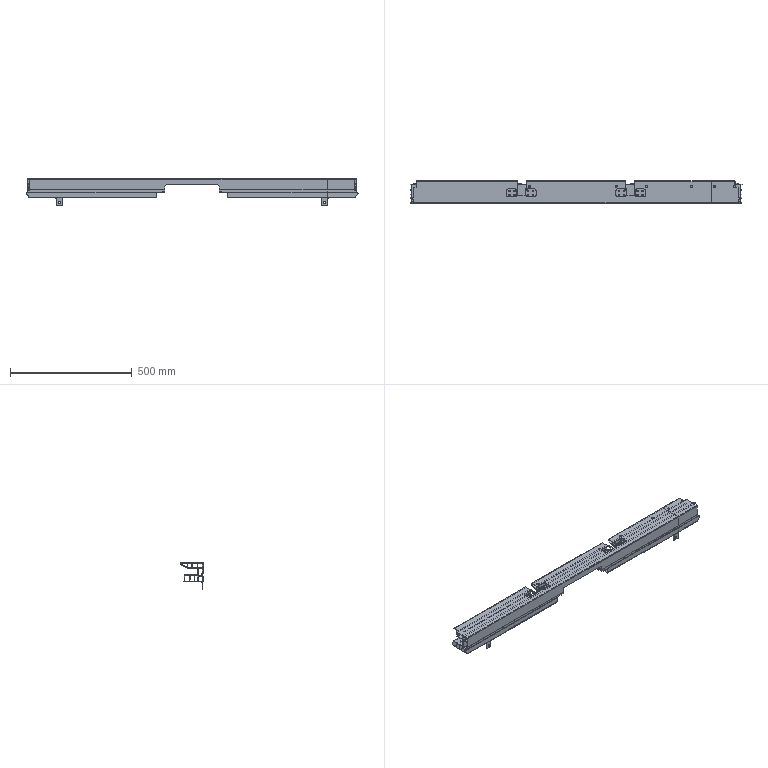NC program | NX | posted with a generic post | part box 1365 x 90.95 x 108.501 mm
Lines 1 to 906 of 22311:
N10 G17 G21 G94 G90
(CAVITY_MILL , TOOL : D16)
N12 T16 M6
N14 G54
N16 G17 G0 G90 X-617.847 Y56.36 B0. C0. S9500 M3
N18 G43 Z30. H16
N20 Z0.503
N22 G94 G1 Z-0.997 F1000.
N24 X-623.563 Y46.46
N26 G2 X-624.429 Y45.96 R1.
N28 G1 X-682.604 F2500.
N30 G3 X-683.352 Y45.208 R0.747
N32 G1 X-683.333 Y41.963
N34 G3 X-682.561 Y41.375 R0.8
N36 G1 X-566.252 Y41.376
N38 G3 X-562.289 Y34.176 R10.036
N40 G1 X-557.527
N42 G2 X-564.365 Y42.175 R8.116
N44 G1 Y45.175
N46 G2 X-557.604 Y53.161 R8.116
N48 G1 X-562.306
N50 G3 X-566.253 Y45.961 R10.036
N52 G1 X-624.429 Y45.96
N54 G2 X-625.295 Y46.46 R1.
N56 G1 X-631.01 Y56.36
N58 Z0.503
N60 G0 X-618.13 Y56.362 Z-0.493
N62 G1 Z-1.993 F1000.
N64 X-623.846 Y46.462
N66 G2 X-624.712 Y45.962 R1.
N68 G1 X-682.604 Y45.961 F2500.
N70 G3 X-683.352 Y45.209 R0.747
N72 G1 X-683.333 Y41.962
N74 G3 X-682.561 Y41.374 R0.8
N76 G1 X-566.819 Y41.375
N78 G3 X-562.862 Y34.175 R10.023
N80 G1 X-558.098
N82 G2 X-564.931 Y42.175 R8.103
N84 G1 Y45.175
N86 G2 X-558.174 Y53.162 R8.103
N88 G1 X-562.879
N90 G3 X-566.82 Y45.962 R10.023
N92 G1 X-624.712
N94 G2 X-625.578 Y46.462 R1.
N96 G1 X-631.294 Y56.362
N98 Z-0.493
N100 G0 X-618.214 Y56.363 Z-1.49
N102 G1 Z-2.99 F1000.
N104 X-623.93 Y46.463
N106 G2 X-624.796 Y45.963 R1.
N108 G1 X-682.604 Y45.962 F2500.
N110 G3 X-683.352 Y45.211 R0.747
N112 G1 X-683.333 Y41.961
N114 G3 X-682.561 Y41.373 R0.8
N116 G1 X-566.986 Y41.374
N118 G3 X-563.03 Y34.174 R10.02
N120 G1 X-558.262
N122 G2 X-565.098 Y42.085 R8.1
N124 G1 X-565.097 Y45.302
N126 G2 X-558.337 Y53.164 R8.099
N128 G1 X-563.047
N130 G3 X-566.987 Y45.964 R10.019
N132 G1 X-624.796 Y45.963
N134 G2 X-625.662 Y46.463 R1.
N136 G1 X-631.378 Y56.363
N138 Z-1.49
N140 G0 X-618.214 Y56.364 Z-2.487
N142 G1 Z-3.987 F1000.
N144 X-623.93 Y46.464
N146 G2 X-624.796 Y45.964 R1.
N148 G1 X-682.604 F2500.
N150 G3 X-683.352 Y45.212 R0.747
N152 G1 X-683.333 Y41.96
N154 G3 X-682.561 Y41.372 R0.8
N156 G1 X-566.987 Y41.373
N158 G3 X-563.03 Y34.173 R10.02
N160 G1 X-558.257
N162 G2 X-565.099 Y42.175 R8.1
N164 G1 Y45.175
N166 G2 X-558.329 Y53.165 R8.1
N168 G1 X-563.046
N170 G3 X-566.988 Y45.965 R10.02
N172 G1 X-624.796 Y45.964
N174 G2 X-625.662 Y46.464 R1.
N176 G1 X-631.378 Y56.364
N178 Z-2.487
N180 G0 X-618.214 Y56.366 Z-3.483
N182 G1 Z-4.983 F1000.
N184 X-623.93 Y46.466
N186 G2 X-624.796 Y45.966 R1.
N188 G1 X-682.604 Y45.965 F2500.
N190 G3 X-683.352 Y45.213 R0.747
N192 G1 X-683.333 Y41.959
N194 G3 X-682.561 Y41.371 R0.8
N196 G1 X-566.987 Y41.372
N198 G3 X-563.029 Y34.172 R10.02
N200 G1 X-558.251
N202 G2 X-565.099 Y42.175 R8.1
N204 G1 Y45.175
N206 G2 X-558.322 Y53.166 R8.1
N208 G1 X-563.044
N210 G3 X-566.988 Y45.966 R10.02
N212 G1 X-624.796
N214 G2 X-625.662 Y46.466 R1.
N216 G1 X-631.378 Y56.365
N218 Z-3.483
N220 G0 X-618.214 Y56.367 Z-4.48
N222 G1 Z-5.98 F1000.
N224 X-623.93 Y46.467
N226 G2 X-624.796 Y45.967 R1.
N228 G1 X-682.604 Y45.966 F2500.
N230 G3 X-683.352 Y45.215 R0.747
N232 G1 X-683.333 Y41.958
N234 G3 X-682.561 Y41.37 R0.8
N236 G1 X-566.987 Y41.371
N238 G3 X-563.027 Y34.171 R10.02
N240 G1 X-558.245
N242 G2 X-565.099 Y42.175 R8.1
N244 G1 Y45.175
N246 G2 X-558.314 Y53.168 R8.1
N248 G1 X-563.042
N250 G3 X-566.988 Y45.968 R10.02
N252 G1 X-624.796 Y45.967
N254 G2 X-625.662 Y46.467 R1.
N256 G1 X-631.378 Y56.367
N258 Z-4.48
N260 G0 X-618.214 Y56.368 Z-5.477
N262 G1 Z-6.977 F1000.
N264 X-623.93 Y46.468
N266 G2 X-624.796 Y45.968 R1.
N268 G1 X-682.604 F2500.
N270 G3 X-683.352 Y45.216 R0.747
N272 G1 X-683.333 Y41.957
N274 G3 X-682.561 Y41.369 R0.8
N276 G1 X-566.987 Y41.37
N278 G3 X-563.026 Y34.17 R10.02
N280 G1 X-558.238
N282 G2 X-565.099 Y42.175 R8.1
N284 G1 Y45.175
N286 G2 X-558.306 Y53.169 R8.1
N288 G1 X-563.04
N290 G3 X-566.988 Y45.969 R10.02
N292 G1 X-624.796 Y45.968
N294 G2 X-625.662 Y46.468 R1.
N296 G1 X-631.378 Y56.368
N298 Z-5.477
N300 G0 X-618.214 Y56.37 Z-6.473
N302 G1 Z-7.973 F1000.
N304 X-623.93 Y46.469
N306 G2 X-624.796 Y45.969 R1.
N308 G1 X-682.604 F2500.
N310 G3 X-683.352 Y45.217 R0.747
N312 G1 X-683.333 Y41.956
N314 G3 X-682.561 Y41.368 R0.8
N316 G1 X-566.987 Y41.369
N318 G3 X-563.025 Y34.169 R10.02
N320 G1 X-558.232
N322 G2 X-565.099 Y42.175 R8.1
N324 G1 Y45.175
N326 G2 X-558.298 Y53.17 R8.1
N328 G1 X-563.039
N330 G3 X-566.988 Y45.97 R10.02
N332 G1 X-624.796 Y45.969
N334 G2 X-625.662 Y46.469 R1.
N336 G1 X-631.378 Y56.369
N338 Z-6.473
N340 G0 X-618.214 Y56.371 Z-7.47
N342 G1 Z-8.97 F1000.
N344 X-623.93 Y46.471
N346 G2 X-624.796 Y45.971 R1.
N348 G1 X-682.604 Y45.97 F2500.
N350 G3 X-683.352 Y45.219 R0.747
N352 G1 X-683.333 Y41.955
N354 G3 X-682.561 Y41.367 R0.8
N356 G1 X-566.987 Y41.368
N358 G3 X-563.024 Y34.168 R10.02
N360 G1 X-558.226
N362 G2 X-565.099 Y42.175 R8.1
N364 G1 Y45.175
N366 G2 X-558.29 Y53.172 R8.1
N368 G1 X-563.037 Y53.171
N370 G3 X-566.987 Y45.971 R10.02
N372 G1 X-624.796
N374 G2 X-625.662 Y46.471 R1.
N376 G1 X-631.378 Y56.371
N378 Z-7.47
N380 G0 X-618.214 Y56.372 Z-8.467
N382 G1 Z-9.967 F1000.
N384 X-623.93 Y46.472
N386 G2 X-624.796 Y45.972 R1.
N388 G1 X-682.604 Y45.971 F2500.
N390 G3 X-683.352 Y45.22 R0.747
N392 G1 X-683.333 Y41.954
N394 G3 X-682.561 Y41.366 R0.8
N396 G1 X-566.987 Y41.367
N398 G3 X-563.022 Y34.167 R10.02
N400 G1 X-558.219
N402 G2 X-565.099 Y42.175 R8.1
N404 G1 Y45.175
N406 G2 X-558.281 Y53.173 R8.1
N408 G1 X-563.035
N410 G3 X-566.987 Y45.973 R10.02
N412 G1 X-624.796 Y45.972
N414 G2 X-625.662 Y46.472 R1.
N416 G1 X-631.378 Y56.372
N418 Z-8.467
N420 G0 X-618.214 Y56.373 Z-9.463
N422 G1 Z-10.963 F1000.
N424 X-623.93 Y46.473
N426 G2 X-624.796 Y45.973 R1.
N428 G1 X-682.604 F2500.
N430 G3 X-683.352 Y45.221 R0.747
N432 G1 X-683.333 Y41.953
N434 G3 X-682.561 Y41.365 R0.8
N436 G1 X-566.986 Y41.366
N438 G3 X-563.021 Y34.166 R10.02
N440 G1 X-558.213
N442 G2 X-565.099 Y42.175 R8.1
N444 G1 Y45.175
N446 G2 X-558.273 Y53.174 R8.1
N448 G1 X-563.034
N450 G3 X-566.987 Y45.974 R10.02
N452 G1 X-624.796 Y45.973
N454 G2 X-625.662 Y46.473 R1.
N456 G1 X-631.378 Y56.373
N458 Z-9.463
N460 G0 X-618.214 Y56.375 Z-10.46
N462 G1 Z-11.96 F1000.
N464 X-623.93 Y46.475
N466 G2 X-624.796 Y45.975 R1.
N468 G1 X-682.604 Y45.974 F2500.
N470 G3 X-683.352 Y45.222 R0.747
N472 G1 X-683.333 Y41.952
N474 G3 X-682.561 Y41.364 R0.8
N476 G1 X-566.986 Y41.365
N478 G3 X-563.02 Y34.165 R10.02
N480 G1 X-558.207 Y34.166
N482 G2 X-565.099 Y42.175 R8.1
N484 G1 Y45.175
N486 G2 X-558.265 Y53.175 R8.1
N488 G1 X-563.032
N490 G3 X-566.987 Y45.975 R10.02
N492 G1 X-624.796
N494 G2 X-625.662 Y46.475 R1.
N496 G1 X-631.378 Y56.375
N498 Z-10.46
N500 G0 X-618.214 Y56.376 Z-11.457
N502 G1 Z-12.957 F1000.
N504 X-623.93 Y46.476
N506 G2 X-624.796 Y45.976 R1.
N508 G1 X-682.604 Y45.975 F2500.
N510 G3 X-683.352 Y45.224 R0.747
N512 G1 X-683.333 Y41.951
N514 G3 X-682.561 Y41.363 R0.8
N516 G1 X-566.986 Y41.364
N518 G3 X-563.018 Y34.164 R10.02
N520 G1 X-558.2 Y34.165
N522 G2 X-565.099 Y42.175 R8.1
N524 G1 Y45.175
N526 G2 X-558.257 Y53.177 R8.1
N528 G1 X-563.03
N530 G3 X-566.987 Y45.977 R10.02
N532 G1 X-624.796 Y45.976
N534 G2 X-625.662 Y46.476 R1.
N536 G1 X-631.378 Y56.376
N538 Z-11.457
N540 G0 X-618.214 Y56.377 Z-12.453
N542 G1 Z-13.953 F1000.
N544 X-623.93 Y46.477
N546 G2 X-624.796 Y45.977 R1.
N548 G1 X-682.604 F2500.
N550 G3 X-683.352 Y45.225 R0.747
N552 G1 X-683.333 Y41.95
N554 G3 X-682.561 Y41.362 R0.8
N556 G1 X-566.986 Y41.363
N558 G3 X-563.017 Y34.164 R10.02
N560 G1 X-558.194
N562 G2 X-565.099 Y42.175 R8.1
N564 G1 Y45.175
N566 G2 X-558.248 Y53.178 R8.1
N568 G1 X-563.028
N570 G3 X-566.987 Y45.978 R10.02
N572 G1 X-624.796 Y45.977
N574 G2 X-625.662 Y46.477 R1.
N576 G1 X-631.377 Y56.377
N578 Z-12.453
N580 G0 X-618.214 Y56.379 Z-13.45
N582 G1 Z-14.95 F1000.
N584 X-623.93 Y46.479
N586 G2 X-624.796 Y45.979 R1.
N588 G1 X-682.604 Y45.978 F2500.
N590 G3 X-683.352 Y45.226 R0.747
N592 G1 X-683.333 Y41.949
N594 G3 X-682.561 Y41.361 R0.8
N596 G1 X-566.986 Y41.363
N598 G3 X-563.016 Y34.163 R10.02
N600 G1 X-558.187
N602 G2 X-565.099 Y42.175 R8.1
N604 G1 Y45.175
N606 G2 X-558.24 Y53.179 R8.1
N608 G1 X-563.027
N610 G3 X-566.987 Y45.979 R10.02
N612 G1 X-624.796
N614 G2 X-625.662 Y46.479 R1.
N616 G1 X-631.377 Y56.379
N618 Z-13.45
N620 G0 X-618.214 Y56.38 Z-14.447
N622 G1 Z-15.947 F1000.
N624 X-623.929 Y46.48
N626 G2 X-624.795 Y45.98 R1.
N628 G1 X-682.604 Y45.979 F2500.
N630 G3 X-683.352 Y45.228 R0.747
N632 G1 X-683.333 Y41.949
N634 G3 X-682.561 Y41.36 R0.8
N636 G1 X-566.986 Y41.362
N638 G3 X-563.015 Y34.162 R10.02
N640 G1 X-558.181
N642 G2 X-565.099 Y42.175 R8.1
N644 G1 Y45.175
N646 G2 X-558.232 Y53.181 R8.1
N648 G1 X-563.025
N650 G3 X-566.987 Y45.981 R10.02
N652 G1 X-624.795 Y45.98
N654 G2 X-625.662 Y46.48 R1.
N656 G1 X-631.377 Y56.38
N658 Z-14.447
N660 G0 X-618.214 Y56.381 Z-15.443
N662 G1 Z-16.943 F1000.
N664 X-623.929 Y46.481
N666 G2 X-624.795 Y45.981 R1.
N668 G1 X-682.604 F2500.
N670 G3 X-683.352 Y45.229 R0.747
N672 G1 X-683.333 Y41.948
N674 G3 X-682.561 Y41.359 R0.8
N676 G1 X-566.986 Y41.361
N678 G3 X-563.013 Y34.161 R10.02
N680 G1 X-558.174
N682 G2 X-565.099 Y42.175 R8.1
N684 G1 Y45.175
N686 G2 X-558.223 Y53.182 R8.1
N688 G1 X-563.023
N690 G3 X-566.987 Y45.982 R10.02
N692 G1 X-624.795 Y45.981
N694 G2 X-625.661 Y46.481 R1.
N696 G1 X-631.377 Y56.381
N698 Z-15.443
N700 G0 X-618.214 Y56.383 Z-16.44
N702 G1 Z-17.94 F1000.
N704 X-623.929 Y46.483
N706 G2 X-624.795 Y45.983 R1.
N708 G1 X-682.604 Y45.982 F2500.
N710 G3 X-683.352 Y45.23 R0.747
N712 G1 X-683.333 Y41.947
N714 G3 X-682.561 Y41.358 R0.8
N716 G1 X-566.986 Y41.36
N718 G3 X-563.012 Y34.16 R10.02
N720 G1 X-558.167
N722 G2 X-565.099 Y42.175 R8.1
N724 G1 Y45.175
N726 G2 X-558.214 Y53.183 R8.1
N728 G1 X-563.021
N730 G3 X-566.986 Y45.983 R10.02
N732 G1 X-624.795
N734 G2 X-625.661 Y46.483 R1.
N736 G1 X-631.377 Y56.382
N738 Z-16.44
N740 G0 X-618.214 Y56.384 Z-17.437
N742 G1 Z-18.937 F1000.
N744 X-623.929 Y46.484
N746 G2 X-624.795 Y45.984 R1.
N748 G1 X-682.604 Y45.983 F2500.
N750 G3 X-683.352 Y45.232 R0.747
N752 G1 X-683.333 Y41.946
N754 G3 X-682.561 Y41.357 R0.8
N756 G1 X-566.986 Y41.359
N758 G3 X-563.011 Y34.159 R10.02
N760 G1 X-558.161
N762 G2 X-565.099 Y42.175 R8.1
N764 G1 Y45.175
N766 G2 X-558.206 Y53.185 R8.1
N768 G1 X-563.02
N770 G3 X-566.986 Y45.985 R10.02
N772 G1 X-624.795 Y45.984
N774 G2 X-625.661 Y46.484 R1.
N776 G1 X-631.377 Y56.384
N778 Z-17.437
N780 G0 X-618.214 Y56.385 Z-18.433
N782 G1 Z-19.933 F1000.
N784 X-623.929 Y46.485
N786 G2 X-624.795 Y45.985 R1.
N788 G1 X-682.604 Y45.984 F2500.
N790 G3 X-683.352 Y45.233 R0.747
N792 G1 X-683.333 Y41.945
N794 G3 X-682.561 Y41.356 R0.8
N796 G1 X-566.986 Y41.358
N798 G3 X-563.009 Y34.158 R10.02
N800 G1 X-558.154
N802 G2 X-565.099 Y42.175 R8.1
N804 G1 Y45.175
N806 G2 X-558.197 Y53.186 R8.1
N808 G1 X-563.018
N810 G3 X-566.986 Y45.986 R10.02
N812 G1 X-624.795 Y45.985
N814 G2 X-625.661 Y46.485 R1.
N816 G1 X-631.377 Y56.385
N818 Z-18.433
N820 G0 X-618.214 Y56.387 Z-19.43
N822 G1 Z-20.93 F1000.
N824 X-623.929 Y46.486
N826 G2 X-624.795 Y45.986 R1.
N828 G1 X-682.604 F2500.
N830 G3 X-683.352 Y45.234 R0.747
N832 G1 X-683.333 Y41.944
N834 G3 X-682.561 Y41.355 R0.8
N836 G1 X-566.986 Y41.357
N838 G3 X-563.008 Y34.157 R10.02
N840 G1 X-558.147
N842 G2 X-565.099 Y42.175 R8.1
N844 G1 Y45.175
N846 G2 X-558.188 Y53.187 R8.1
N848 G1 X-563.016
N850 G3 X-566.986 Y45.987 R10.02
N852 G1 X-624.795 Y45.986
N854 G2 X-625.661 Y46.486 R1.
N856 G1 X-631.377 Y56.386
N858 Z-19.43
N860 G0 X-618.213 Y56.388 Z-20.427
N862 G1 Z-21.927 F1000.
N864 X-623.929 Y46.488
N866 G2 X-624.795 Y45.988 R1.
N868 G1 X-682.604 Y45.987 F2500.
N870 G3 X-683.352 Y45.236 R0.747
N872 G1 X-683.333 Y41.943
N874 G3 X-682.561 Y41.354 R0.8
N876 G1 X-566.986 Y41.356
N878 G3 X-563.007 Y34.156 R10.02
N880 G1 X-558.14
N882 G2 X-565.099 Y42.175 R8.1
N884 G1 Y45.175
N886 G2 X-558.18 Y53.189 R8.1
N888 G1 X-563.014 Y53.188
N890 G3 X-566.986 Y45.988 R10.02
N892 G1 X-624.795
N894 G2 X-625.661 Y46.488 R1.
N896 G1 X-631.377 Y56.388
N898 Z-20.427
N900 G0 X-618.213 Y56.389 Z-21.423
N902 G1 Z-22.923 F1000.
N904 X-623.929 Y46.489
N906 G2 X-624.795 Y45.989 R1.
N908 G1 X-682.604 Y45.988 F2500.
N910 G3 X-683.352 Y45.237 R0.747
N912 G1 X-683.333 Y41.942
N914 G3 X-682.561 Y41.353 R0.8
N916 G1 X-566.985 Y41.355
N918 G3 X-563.005 Y34.155 R10.02
N920 G1 X-558.134
N922 G2 X-565.099 Y42.175 R8.1
N924 G1 Y45.175
N926 G2 X-558.171 Y53.19 R8.1
N928 G1 X-563.013
N930 G3 X-566.986 Y45.99 R10.02
N932 G1 X-624.795 Y45.989
N934 G2 X-625.661 Y46.489 R1.
N936 G1 X-631.377 Y56.389
N938 Z-21.423
N940 G0 X-618.213 Y56.39 Z-22.42
N942 G1 Z-23.92 F1000.
N944 X-623.929 Y46.49
N946 G2 X-624.795 Y45.99 R1.
N948 G1 X-682.604 F2500.
N950 G3 X-683.352 Y45.238 R0.747
N952 G1 X-683.333 Y41.941
N954 G3 X-682.561 Y41.352 R0.8
N956 G1 X-566.985 Y41.354
N958 G3 X-563.004 Y34.154 R10.02
N960 G1 X-558.127
N962 G2 X-565.099 Y42.175 R8.1
N964 G1 Y45.175
N966 G2 X-558.162 Y53.191 R8.1
N968 G1 X-563.011
N970 G3 X-566.986 Y45.991 R10.02
N972 G1 X-624.795 Y45.99
N974 G2 X-625.661 Y46.49 R1.
N976 G1 X-631.377 Y56.39
N978 Z-22.42
N980 G0 X-618.213 Y56.392 Z-23.417
N982 G1 Z-24.917 F1000.
N984 X-623.929 Y46.492
N986 G2 X-624.795 Y45.992 R1.
N988 G1 X-682.604 Y45.991 F2500.
N990 G3 X-683.352 Y45.239 R0.747
N992 G1 X-683.333 Y41.94
N994 G3 X-682.561 Y41.351 R0.8
N996 G1 X-566.985 Y41.353
N998 G3 X-563.003 Y34.153 R10.02
N1000 G1 X-558.12
N1002 G2 X-565.099 Y42.175 R8.1
N1004 G1 Y45.175
N1006 G2 X-558.153 Y53.192 R8.1
N1008 G1 X-563.009
N1010 G3 X-566.986 Y45.992 R10.02
N1012 G1 X-624.795
N1014 G2 X-625.661 Y46.492 R1.
N1016 G1 X-631.377 Y56.392
N1018 Z-23.417
N1020 G0 X-618.257 Y56.393 Z-24.413
N1022 G1 Z-25.913 F1000.
N1024 X-623.973 Y46.493
N1026 G2 X-624.839 Y45.993 R1.
N1028 G1 X-682.604 Y45.992 F2500.
N1030 G3 X-683.352 Y45.241 R0.747
N1032 G1 X-683.333 Y41.833
N1034 G3 X-682.561 Y41.245 R0.8
N1036 G1 X-567.072 Y41.246
N1038 G3 X-563.08 Y34.046 R9.992
N1040 G1 X-558.073
N1042 G2 X-565.185 Y42.084 R8.072
N1044 G1 Y45.175
N1046 G2 X-558.28 Y53.194 R8.081
N1048 G1 X-563.112
N1050 G3 X-567.073 Y45.994 R10.001
N1052 G1 X-624.839 Y45.993
N1054 G2 X-625.705 Y46.493 R1.
N1056 G1 X-631.421 Y56.393
N1058 Z-24.413
N1060 G0 X-618.421 Y56.394 Z-25.41
N1062 G1 Z-26.91 F1000.
N1064 X-624.137 Y46.494
N1066 G2 X-625.003 Y45.994 R1.
N1068 G1 X-682.604 F2500.
N1070 G3 X-683.352 Y45.242 R0.748
N1072 G1 X-683.333 Y41.583
N1074 G3 X-682.561 Y40.995 R0.8
N1076 G1 X-567.402 Y40.997
N1078 G3 X-567.25 Y39.987 R4.779
N1080 X-563.458 Y33.797 R9.98
N1082 G1 X-558.749
N1084 G2 X-565.374 Y40.407 R8.06
N1086 X-565.487 Y41.203 R2.859
N1088 G1 Y45.175
N1090 X-565.519 Y45.302
N1092 G2 X-561.523 Y52.155 R8.234
N1094 X-558.598 Y53.195 R7.861
N1096 G1 X-563.41
N1098 G3 X-567.402 Y45.995 R10.154
N1100 G1 X-625.003 Y45.994
N1102 G2 X-625.869 Y46.494 R1.
N1104 G1 X-631.585 Y56.394
N1106 Z-25.41
N1108 G0 X-618.711 Y56.396 Z-26.407
N1110 G1 Z-27.907 F1000.
N1112 X-624.426 Y46.496
N1114 G2 X-625.292 Y45.996 R1.
N1116 G1 X-682.604 Y45.995 F2500.
N1118 G3 X-683.352 Y45.243 R0.748
N1120 G1 X-683.332 Y41.013
N1122 G3 X-682.561 Y40.427 R0.8
N1124 G1 X-567.948 Y40.428
N1126 G3 X-564.041 Y33.228 R9.956
N1128 G1 X-559.333
N1130 G2 X-566.054 Y41.156 R8.036
N1132 G1 Y45.175
N1134 X-566.097 Y45.302
N1136 G2 X-559.08 Y53.196 R8.148
N1138 G1 X-563.972
N1140 G3 X-567.981 Y45.996 R10.068
N1142 G1 X-625.292
N1144 G2 X-626.158 Y46.496 R1.
N1146 G1 X-631.874 Y56.396
N1148 Z-26.407
N1150 G0 X-619.185 Y56.397 Z-27.403
N1152 G1 Z-28.903 F1000.
N1154 X-624.901 Y46.497
N1156 G2 X-625.767 Y45.997 R1.
N1158 G1 X-682.604 Y45.996 F2500.
N1160 G3 X-683.352 Y45.245 R0.749
N1162 G1 X-683.332 Y40.048
N1164 G3 X-682.561 Y39.462 R0.8
N1166 G1 X-568.93 Y39.464
N1168 G3 X-565.034 Y32.264 R9.977
N1170 G1 X-560.403
N1172 G2 X-567.037 Y40.194 R8.057
N1174 G1 Y45.175
N1176 G2 X-561.439 Y52.88 R7.978
N1178 X-560.005 Y53.198 R8.728
N1180 G1 X-564.98
N1182 G3 X-568.93 Y45.998 R9.898
N1184 G1 X-625.767 Y45.997
N1186 G2 X-626.633 Y46.497 R1.
N1188 G1 X-632.349 Y56.397
N1190 Z-27.403
N1192 G0 X-620.523 Y56.398 Z-28.4
N1194 G1 Z-29.9 F1000.
N1196 X-626.239 Y46.498
N1198 G2 X-627.105 Y45.998 R1.
N1200 G1 X-682.603 F2500.
N1202 G3 X-683.353 Y45.246 R0.749
N1204 G1 X-683.331 Y37.752
N1206 G3 X-682.561 Y37.168 R0.8
N1208 G1 X-571.644 Y37.169
N1210 G3 X-568.245 Y29.969 R9.925
N1212 G1 X-564.571 Y29.97
N1214 G2 X-569.728 Y37.451 R8.005
N1216 G1 Y45.23
N1218 G2 X-562.78 Y53.199 R8.235
N1220 G1 X-567.574
N1222 G3 X-571.607 Y45.999 R10.155
N1224 G1 X-627.105 Y45.998
N1226 G2 X-627.971 Y46.498 R1.
N1228 G1 X-633.687 Y56.398
N1230 Z-28.4
N1232 G0 X-670.093 Y56.703 Z-29.32
N1234 G1 Z-30.82 F1000.
N1236 X-671.677 Y53.959
N1238 G2 X-672.543 Y53.459 R1.
N1240 G1 X-674.899 F2500.
N1242 G3 X-678.862 Y46.259 R10.063
N1244 G1 X-682.602
N1246 G3 X-683.353 Y45.508 R0.751
N1248 G1 X-683.338 Y-35.817
N1250 G3 X-682.561 Y-36.425 R0.8
N1252 G1 X-677.313
N1254 G3 X-674.709 Y-40.867 R10.168
N1256 G1 X-672.866 Y-42.71
N1258 G3 X-671.814 Y-43.625 R10.02
N1260 G1 X-667.051
N1262 G2 X-671.508 Y-41.353 R8.1
N1264 G1 X-673.352 Y-39.509
N1266 G2 X-675.724 Y-34.564 R8.248
N1268 X-676.977 Y-30.247 R7.901
N1270 G1 Y45.461
N1272 G2 X-670.187 Y53.46 R8.143
N1274 G1 X-672.543 Y53.459
N1276 G2 X-673.409 Y53.959 R1.
N1278 G1 X-674.968 Y56.659
N1280 Z-29.32
N1282 G0 X-670.102 Y56.688 Z-30.24
N1284 G1 Z-31.74 F1000.
N1286 X-671.677 Y53.959
N1288 G2 X-672.543 Y53.459 R1.
N1290 G1 X-675.029 F2500.
N1292 G3 X-679.175 Y47.418 R10.791
N1294 X-679.425 Y46.259 R13.842
N1296 G1 X-682.602
N1298 G3 X-683.353 Y45.508 R0.751
N1300 G1 X-683.338 Y-35.817
N1302 G3 X-682.561 Y-36.425 R0.8
N1304 G1 X-677.384
N1306 X-677.282 Y-36.548
N1308 G3 X-674.708 Y-40.868 R10.182
N1310 G1 X-672.866 Y-42.71
N1312 G3 X-671.814 Y-43.625 R10.02
N1314 G1 X-667.051
N1316 G2 X-671.508 Y-41.353 R8.1
N1318 G1 X-673.352 Y-39.509
N1320 G2 X-675.546 Y-35.613 R8.262
N1322 X-677.703 Y-30.125 R8.043
N1324 G1 Y43.975
N1326 G2 X-677.317 Y46.934 R11.922
N1328 X-670.104 Y53.46 R8.871
N1330 G1 X-672.543 Y53.459
N1332 G2 X-673.409 Y53.959 R1.
N1334 G1 X-674.968 Y56.659
N1336 Z-30.24
N1338 G0 X-670.095 Y56.7 Z-31.16
N1340 G1 Z-32.66 F1000.
N1342 X-671.677 Y53.959
N1344 G2 X-672.543 Y53.459 R1.
N1346 G1 X-675.039 F2500.
N1348 G3 X-677.529 Y50.937 R10.732
N1350 X-680.085 Y46.259 R10.007
N1352 G1 X-682.602
N1354 G3 X-683.353 Y45.508 R0.751
N1356 G1 X-683.338 Y-35.746
N1358 G3 X-682.561 Y-36.354 R0.8
N1360 G1 X-678.173
N1362 G3 X-676.866 Y-37.712 R10.011
N1364 X-674.708 Y-40.868 R10.294
N1366 G1 X-672.866 Y-42.71
N1368 G3 X-671.907 Y-43.554 R10.02
N1370 G1 X-667.435
N1372 G2 X-671.508 Y-41.353 R8.1
N1374 G1 X-673.352 Y-39.509
N1376 G2 X-675.273 Y-36.534 R8.374
N1378 G1 X-675.331 Y-36.489
N1380 G2 X-678.429 Y-30.125 R8.091
N1382 G1 Y-29.243
N1384 G2 X-678.276 Y-27.678 R6.48
N1386 G1 Y-11.514
N1388 G2 X-678.429 Y-9.914 R7.58
N1390 G1 Y-7.068
N1392 G2 X-678.276 Y-5.551 R7.564
N1394 G1 Y6.994
N1396 X-678.302 Y7.121
N1398 X-678.43 Y8.301
N1400 X-678.429 Y8.586
N1402 Y12.068
N1404 G2 X-678.276 Y13.642 R7.063
N1406 G1 Y19.281
N1408 G2 X-678.429 Y20.882 R7.729
N1410 G1 Y26.068
N1412 G2 X-678.276 Y27.676 R8.328
N1414 G1 Y41.039
N1416 G2 X-678.429 Y42.586 R6.069
N1418 G1 Y43.975
N1420 G2 X-676.045 Y49.708 R8.087
N1422 X-670.173 Y53.46 R8.812
N1424 G1 X-672.543 Y53.459
N1426 G2 X-673.409 Y53.959 R1.
N1428 G1 X-674.968 Y56.659
N1430 Z-31.16
N1432 G0 X-670.075 Y56.735 Z-32.08
N1434 G1 Z-33.58 F1000.
N1436 X-671.677 Y53.959
N1438 G2 X-672.543 Y53.459 R1.
N1440 G1 X-675.189 F2500.
N1442 X-675.331 Y53.35
N1444 X-677.243 Y51.849
N1446 G3 X-680.811 Y46.259 R10.011
N1448 G1 X-682.719
N1450 G3 X-683.337 Y45.67 R0.8
N1452 G1 X-683.331 Y42.215
N1454 G3 X-682.719 Y41.649 R0.8
N1456 G1 X-680.987
N1458 G3 X-680.196 Y38.871 R10.038
N1460 G1 Y34.449
N1462 X-678.276
N1464 Y39.305
N1466 G2 X-679.156 Y42.975 R8.118
N1468 G1 Y43.975
N1470 G2 X-676.058 Y50.339 R8.091
N1472 G1 X-674.146 Y51.839
N1474 G2 X-670.487 Y53.459 R8.145
N1476 G1 X-672.543
N1478 G2 X-673.409 Y53.959 R1.
N1480 G1 X-674.968 Y56.659
N1482 Z-32.08
N1484 G0 X-670.053 Y56.773 Z-33.
N1486 G1 Z-34.5 F1000.
N1488 X-671.677 Y53.959
N1490 G2 X-672.543 Y53.459 R1.
N1492 G1 X-675.915 F2500.
N1494 X-676.058 Y53.35
N1496 X-677.969 Y51.849
N1498 G3 X-681.537 Y46.259 R10.011
N1500 G1 X-682.605
N1502 G3 X-683.351 Y45.508 R0.747
N1504 G1 X-683.333 Y42.745
N1506 G3 X-682.561 Y42.155 R0.8
N1508 G1 X-681.768
N1510 G3 X-680.196 Y37.539 R10.023
N1512 G1 Y34.955
N1514 X-678.276
N1516 Y38.138
N1518 G2 X-679.882 Y42.975 R8.103
N1520 G1 Y43.976
N1522 G2 X-676.784 Y50.339 R8.091
N1524 G1 X-674.873 Y51.839
N1526 G2 X-671.213 Y53.459 R8.145
N1528 G1 X-672.543
N1530 G2 X-673.409 Y53.959 R1.
N1532 G1 X-674.968 Y56.659
N1534 Z-33.
N1536 G0 X-670.051 Y56.775 Z-33.968
N1538 G1 Z-35.468 F1000.
N1540 X-671.677 Y53.959
N1542 G2 X-672.543 Y53.459 R1.
N1544 G1 X-676.679 F2500.
N1546 X-676.823 Y53.349
N1548 X-678.734 Y51.849
N1550 G3 X-682.302 Y46.259 R10.011
N1552 G1 X-682.605
N1554 G3 X-683.351 Y45.508 R0.747
N1556 G1 X-683.333 Y42.745
N1558 G3 X-682.532 Y42.155 R0.801
N1560 X-680.196 Y36.503 R10.061
N1562 G1 Y34.955
N1564 X-678.276
N1566 Y37.248
N1568 G2 X-680.646 Y42.975 R8.141
N1570 G1 Y43.975
N1572 G2 X-677.548 Y50.339 R8.091
N1574 G1 X-675.637 Y51.839
N1576 G2 X-671.955 Y53.459 R8.231
N1578 G1 X-672.543
N1580 G2 X-673.409 Y53.959 R1.
N1582 G1 X-674.968 Y56.659
N1584 Z-33.968
N1586 G0 X-676.003 Z-34.937
N1588 G1 Z-36.437 F1000.
N1590 X-673.645 Y53.808
N1592 G3 X-672.708 Y53.459 R1.
N1594 G1 X-677.443 F2500.
N1596 X-677.587 Y53.349
N1598 X-679.498 Y51.849
N1600 G3 X-683.11 Y46.062 R10.011
N1602 X-683.351 Y45.508 R0.747
N1604 G1 X-683.333 Y42.745
N1606 X-683.327 Y42.725
N1608 G3 X-680.196 Y35.699 R10.044
N1610 G1 Y34.955
N1612 X-678.276
N1614 Y36.578
N1616 G2 X-681.411 Y42.975 R8.124
N1618 G1 Y43.975
N1620 G2 X-678.313 Y50.339 R8.091
N1622 G1 X-676.402 Y51.839
N1624 G2 X-672.708 Y53.459 R8.278
N1626 G3 X-671.937 Y54.097 R1.
N1628 G1 X-670.941 Y56.775
N1630 Z-34.937
N1632 G0 X-676.777 Y56.659 Z-35.905
N1634 G1 Z-37.405 F1000.
N1636 X-674.418 Y53.808
N1638 G3 X-673.481 Y53.459 R1.
N1640 G1 X-678.208 F2500.
N1642 X-678.352 Y53.349
N1644 X-680.263 Y51.849
N1646 G3 X-684.096 Y43.976 R10.011
N1648 G1 Y42.975
N1650 G3 X-680.196 Y35.051 R10.006
N1652 G1 Y34.955
N1654 X-680.068
N1656 X-678.944
N1658 X-678.276
N1660 Y36.06
N1662 G2 X-682.176 Y42.975 R8.086
N1664 G1 Y43.975
N1666 G2 X-679.078 Y50.339 R8.091
N1668 G1 X-677.166 Y51.839
N1670 G2 X-673.481 Y53.459 R8.246
N1672 G3 X-672.71 Y54.097 R1.
N1674 G1 X-671.715 Y56.775
N1676 Z-35.905
N1678 G0 Z30.
N1680 X-681.658 Y33.981
N1682 Z-36.874
N1684 G1 Z-38.374 F1000.
N1686 X-678.343 Y34.704
N1688 G3 X-678.276 Y34.954 R0.5
N1690 G1 Y35.647 F2500.
N1692 G2 X-682.94 Y42.975 R8.179
N1694 G1 Y43.975
N1696 G2 X-679.842 Y50.339 R8.091
N1698 G1 X-677.931 Y51.839
N1700 G2 X-674.237 Y53.459 R8.277
N1702 G3 X-673.467 Y54.097 R1.
N1704 G1 X-672.47 Y56.775
N1706 Z-36.874
N1708 G0 Z30.
N1710 X-682.429 Y33.976
N1712 Z-37.842
N1714 G1 Z-39.342 F1000.
N1716 X-678.343 Y34.704
N1718 G3 X-678.276 Y34.954 R0.5
N1720 G1 Y35.334 F2500.
N1722 G2 X-683.705 Y42.975 R8.108
N1724 G1 Y43.975
N1726 G2 X-680.607 Y50.339 R8.091
N1728 G1 X-678.695 Y51.839
N1730 G2 X-675.036 Y53.459 R8.145
N1732 G3 X-674.266 Y54.098 R1.
N1734 G1 X-673.274 Y56.775
N1736 Z-37.842
N1738 G0 Z30.
N1740 X-683.191 Y33.975
N1742 Z-38.811
N1744 G1 Z-40.311 F1000.
N1746 X-678.343 Y34.704
N1748 G3 X-678.276 Y34.954 R0.5
N1750 G1 Y35.108 F2500.
N1752 G2 X-684.469 Y42.975 R8.107
N1754 G1 Y43.975
N1756 G2 X-681.371 Y50.339 R8.091
N1758 G1 X-679.46 Y51.839
N1760 G2 X-675.767 Y53.459 R8.278
N1762 G3 X-674.996 Y54.097 R1.
N1764 G1 X-673.999 Y56.775
N1766 Z-38.811
N1768 G0 Z30.
N1770 X-684.911 Y40.617
N1772 Z-38.811
N1774 G1 X-684.245 Y39.044 Z-39.268 F1000.
N1776 X-683.271 Y37.651 Z-39.724
N1778 X-682.029 Y36.492 Z-40.179
N1780 X-680.573 Y35.615 Z-40.634
N1782 X-678.966 Y35.06 Z-41.09
N1784 X-678.276 Y34.962 Z-41.277
N1786 Y34.953 Z-41.279
N1788 Y34.962 F2500.
N1790 G2 X-685.234 Y42.975 R8.105
N1792 G1 Y43.975
N1794 G2 X-682.136 Y50.339 R8.091
N1796 G1 X-680.225 Y51.839
N1798 G2 X-676.531 Y53.459 R8.278
N1800 G3 X-675.76 Y54.097 R1.
N1802 G1 X-674.764 Y56.775
N1804 Z-39.779
N1806 G0 Z30.
N1808 X-684.71 Y33.967
N1810 Z-40.747